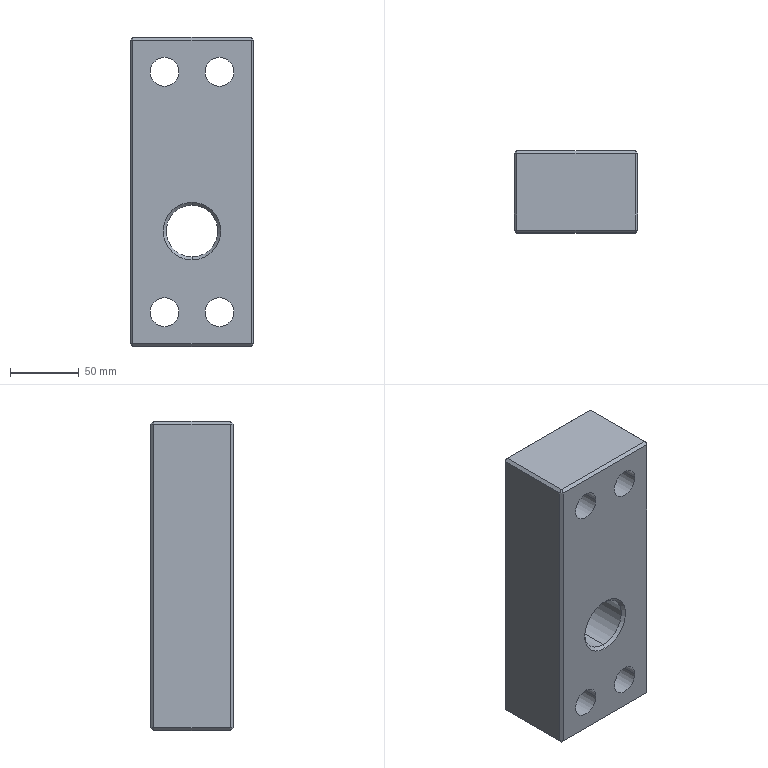Part | Creo | 1 solid | 52 faces | box 90 x 60 x 225 mm | volume 1027341 mm3 | plane 30 | cylinder 18 | cone 4 | commonest cylinder face diameters 21 x8 31 x8 37.616 x2
STEP:
#1=CARTESIAN_POINT('',(43.,400.,103.5));
#2=VERTEX_POINT('',#1);
#3=CARTESIAN_POINT('',(43.,400.,-117.5));
#4=VERTEX_POINT('',#3);
#5=CARTESIAN_POINT('',(43.,400.,103.5));
#6=DIRECTION('',(0.,0.,-1.));
#7=VECTOR('',#6,221.);
#8=LINE('',#5,#7);
#9=EDGE_CURVE('',#2,#4,#8,.T.);
#10=ORIENTED_EDGE('',*,*,#9,.T.);
#11=CARTESIAN_POINT('',(-43.,400.,-117.5));
#12=VERTEX_POINT('',#11);
#13=CARTESIAN_POINT('',(43.,400.,-117.5));
#14=DIRECTION('',(-1.,0.,0.));
#15=VECTOR('',#14,86.);
#16=LINE('',#13,#15);
#17=EDGE_CURVE('',#4,#12,#16,.T.);
#18=ORIENTED_EDGE('',*,*,#17,.T.);
#19=CARTESIAN_POINT('',(-43.,400.,103.5));
#20=VERTEX_POINT('',#19);
#21=CARTESIAN_POINT('',(-43.,400.,-117.5));
#22=DIRECTION('',(0.,0.,1.));
#23=VECTOR('',#22,221.);
#24=LINE('',#21,#23);
#25=EDGE_CURVE('',#12,#20,#24,.T.);
#26=ORIENTED_EDGE('',*,*,#25,.T.);
#27=CARTESIAN_POINT('',(-43.,400.,103.5));
#28=DIRECTION('',(1.,0.,0.));
#29=VECTOR('',#28,86.);
#30=LINE('',#27,#29);
#31=EDGE_CURVE('',#20,#2,#30,.T.);
#32=ORIENTED_EDGE('',*,*,#31,.T.);
#33=EDGE_LOOP('',(#10,#18,#26,#32));
#34=FACE_OUTER_BOUND('',#33,.F.);
#35=CARTESIAN_POINT('',(-30.5,400.,80.5));
#36=VERTEX_POINT('',#35);
#37=CARTESIAN_POINT('',(-9.5,400.,80.5));
#38=VERTEX_POINT('',#37);
#39=CARTESIAN_POINT('',(-20.,400.,80.5));
#40=DIRECTION('',(0.,1.,0.));
#41=DIRECTION('',(-1.,0.,0.));
#42=AXIS2_PLACEMENT_3D('',#39,#40,#41);
#43=CIRCLE('',#42,10.5);
#44=EDGE_CURVE('',#36,#38,#43,.T.);
#45=ORIENTED_EDGE('',*,*,#44,.F.);
#46=CARTESIAN_POINT('',(-20.,400.,80.5));
#47=DIRECTION('',(0.,1.,0.));
#48=DIRECTION('',(1.,0.,0.));
#49=AXIS2_PLACEMENT_3D('',#46,#47,#48);
#50=CIRCLE('',#49,10.5);
#51=EDGE_CURVE('',#38,#36,#50,.T.);
#52=ORIENTED_EDGE('',*,*,#51,.F.);
#53=EDGE_LOOP('',(#45,#52));
#54=FACE_BOUND('',#53,.F.);
#55=CARTESIAN_POINT('',(9.5,400.,-94.5));
#56=VERTEX_POINT('',#55);
#57=CARTESIAN_POINT('',(30.5,400.,-94.5));
#58=VERTEX_POINT('',#57);
#59=CARTESIAN_POINT('',(20.,400.,-94.5));
#60=DIRECTION('',(0.,1.,0.));
#61=DIRECTION('',(-1.,0.,0.));
#62=AXIS2_PLACEMENT_3D('',#59,#60,#61);
#63=CIRCLE('',#62,10.5);
#64=EDGE_CURVE('',#56,#58,#63,.T.);
#65=ORIENTED_EDGE('',*,*,#64,.F.);
#66=CARTESIAN_POINT('',(20.,400.,-94.5));
#67=DIRECTION('',(0.,1.,0.));
#68=DIRECTION('',(1.,0.,0.));
#69=AXIS2_PLACEMENT_3D('',#66,#67,#68);
#70=CIRCLE('',#69,10.5);
#71=EDGE_CURVE('',#58,#56,#70,.T.);
#72=ORIENTED_EDGE('',*,*,#71,.F.);
#73=EDGE_LOOP('',(#65,#72));
#74=FACE_BOUND('',#73,.F.);
#75=CARTESIAN_POINT('',(0.,400.,-56.5));
#76=VERTEX_POINT('',#75);
#77=CARTESIAN_POINT('',(0.,400.,-14.5));
#78=VERTEX_POINT('',#77);
#79=CARTESIAN_POINT('',(0.,400.,-35.5));
#80=DIRECTION('',(0.,1.,0.));
#81=DIRECTION('',(0.,0.,-1.));
#82=AXIS2_PLACEMENT_3D('',#79,#80,#81);
#83=CIRCLE('',#82,21.);
#84=EDGE_CURVE('',#76,#78,#83,.T.);
#85=ORIENTED_EDGE('',*,*,#84,.F.);
#86=CARTESIAN_POINT('',(0.,400.,-35.5));
#87=DIRECTION('',(0.,1.,0.));
#88=DIRECTION('',(0.,0.,1.));
#89=AXIS2_PLACEMENT_3D('',#86,#87,#88);
#90=CIRCLE('',#89,21.);
#91=EDGE_CURVE('',#78,#76,#90,.T.);
#92=ORIENTED_EDGE('',*,*,#91,.F.);
#93=EDGE_LOOP('',(#85,#92));
#94=FACE_BOUND('',#93,.F.);
#95=CARTESIAN_POINT('',(9.5,400.,80.5));
#96=VERTEX_POINT('',#95);
#97=CARTESIAN_POINT('',(30.5,400.,80.5));
#98=VERTEX_POINT('',#97);
#99=CARTESIAN_POINT('',(20.,400.,80.5));
#100=DIRECTION('',(0.,1.,0.));
#101=DIRECTION('',(-1.,0.,0.));
#102=AXIS2_PLACEMENT_3D('',#99,#100,#101);
#103=CIRCLE('',#102,10.5);
#104=EDGE_CURVE('',#96,#98,#103,.T.);
#105=ORIENTED_EDGE('',*,*,#104,.F.);
#106=CARTESIAN_POINT('',(20.,400.,80.5));
#107=DIRECTION('',(0.,1.,0.));
#108=DIRECTION('',(1.,0.,0.));
#109=AXIS2_PLACEMENT_3D('',#106,#107,#108);
#110=CIRCLE('',#109,10.5);
#111=EDGE_CURVE('',#98,#96,#110,.T.);
#112=ORIENTED_EDGE('',*,*,#111,.F.);
#113=EDGE_LOOP('',(#105,#112));
#114=FACE_BOUND('',#113,.F.);
#115=CARTESIAN_POINT('',(-30.5,400.,-94.5));
#116=VERTEX_POINT('',#115);
#117=CARTESIAN_POINT('',(-9.5,400.,-94.5));
#118=VERTEX_POINT('',#117);
#119=CARTESIAN_POINT('',(-20.,400.,-94.5));
#120=DIRECTION('',(0.,1.,0.));
#121=DIRECTION('',(-1.,0.,0.));
#122=AXIS2_PLACEMENT_3D('',#119,#120,#121);
#123=CIRCLE('',#122,10.5);
#124=EDGE_CURVE('',#116,#118,#123,.T.);
#125=ORIENTED_EDGE('',*,*,#124,.F.);
#126=CARTESIAN_POINT('',(-20.,400.,-94.5));
#127=DIRECTION('',(0.,1.,0.));
#128=DIRECTION('',(1.,0.,0.));
#129=AXIS2_PLACEMENT_3D('',#126,#127,#128);
#130=CIRCLE('',#129,10.5);
#131=EDGE_CURVE('',#118,#116,#130,.T.);
#132=ORIENTED_EDGE('',*,*,#131,.F.);
#133=EDGE_LOOP('',(#125,#132));
#134=FACE_BOUND('',#133,.F.);
#135=CARTESIAN_POINT('',(0.,400.,-120.5));
#136=DIRECTION('',(0.,-1.,0.));
#137=DIRECTION('',(0.,0.,-1.));
#138=AXIS2_PLACEMENT_3D('',#135,#136,#137);
#139=PLANE('',#138);
#140=ADVANCED_FACE('',(#34,#54,#74,#94,#114,#134),#139,.T.);
#141=CARTESIAN_POINT('',(30.5,439.,-94.5));
#142=VERTEX_POINT('',#141);
#143=CARTESIAN_POINT('',(9.5,439.,-94.5));
#144=VERTEX_POINT('',#143);
#145=CARTESIAN_POINT('',(20.,439.,-94.5));
#146=DIRECTION('',(0.,-1.,0.));
#147=DIRECTION('',(1.,0.,0.));
#148=AXIS2_PLACEMENT_3D('',#145,#146,#147);
#149=CIRCLE('',#148,10.5);
#150=EDGE_CURVE('',#142,#144,#149,.T.);
#151=ORIENTED_EDGE('',*,*,#150,.T.);
#152=CARTESIAN_POINT('',(9.5,400.,-94.5));
#153=DIRECTION('',(0.,1.,0.));
#154=VECTOR('',#153,39.);
#155=LINE('',#152,#154);
#156=EDGE_CURVE('',#56,#144,#155,.T.);
#157=ORIENTED_EDGE('',*,*,#156,.F.);
#158=ORIENTED_EDGE('',*,*,#64,.T.);
#159=CARTESIAN_POINT('',(30.5,400.,-94.5));
#160=DIRECTION('',(0.,1.,0.));
#161=VECTOR('',#160,39.);
#162=LINE('',#159,#161);
#163=EDGE_CURVE('',#58,#142,#162,.T.);
#164=ORIENTED_EDGE('',*,*,#163,.T.);
#165=EDGE_LOOP('',(#151,#157,#158,#164));
#166=FACE_OUTER_BOUND('',#165,.F.);
#167=CARTESIAN_POINT('',(20.,400.,-94.5));
#168=DIRECTION('',(0.,1.,0.));
#169=DIRECTION('',(-1.,0.,0.));
#170=AXIS2_PLACEMENT_3D('',#167,#168,#169);
#171=CYLINDRICAL_SURFACE('',#170,10.5);
#172=ADVANCED_FACE('',(#166),#171,.F.);
#173=CARTESIAN_POINT('',(4.5,439.,-94.5));
#174=VERTEX_POINT('',#173);
#175=CARTESIAN_POINT('',(35.5,439.,-94.5));
#176=VERTEX_POINT('',#175);
#177=CARTESIAN_POINT('',(20.,439.,-94.5));
#178=DIRECTION('',(0.,1.,0.));
#179=DIRECTION('',(-1.,0.,0.));
#180=AXIS2_PLACEMENT_3D('',#177,#178,#179);
#181=CIRCLE('',#180,15.5);
#182=EDGE_CURVE('',#174,#176,#181,.T.);
#183=ORIENTED_EDGE('',*,*,#182,.F.);
#184=CARTESIAN_POINT('',(20.,439.,-94.5));
#185=DIRECTION('',(0.,1.,0.));
#186=DIRECTION('',(1.,0.,0.));
#187=AXIS2_PLACEMENT_3D('',#184,#185,#186);
#188=CIRCLE('',#187,15.5);
#189=EDGE_CURVE('',#176,#174,#188,.T.);
#190=ORIENTED_EDGE('',*,*,#189,.F.);
#191=EDGE_LOOP('',(#183,#190));
#192=FACE_OUTER_BOUND('',#191,.F.);
#193=CARTESIAN_POINT('',(20.,439.,-94.5));
#194=DIRECTION('',(0.,-1.,0.));
#195=DIRECTION('',(-1.,0.,0.));
#196=AXIS2_PLACEMENT_3D('',#193,#194,#195);
#197=CIRCLE('',#196,10.5);
#198=EDGE_CURVE('',#144,#142,#197,.T.);
#199=ORIENTED_EDGE('',*,*,#198,.F.);
#200=ORIENTED_EDGE('',*,*,#150,.F.);
#201=EDGE_LOOP('',(#199,#200));
#202=FACE_BOUND('',#201,.F.);
#203=CARTESIAN_POINT('',(20.,439.,-94.5));
#204=DIRECTION('',(0.,-1.,0.));
#205=DIRECTION('',(1.,0.,0.));
#206=AXIS2_PLACEMENT_3D('',#203,#204,#205);
#207=PLANE('',#206);
#208=ADVANCED_FACE('',(#192,#202),#207,.F.);
#209=ORIENTED_EDGE('',*,*,#198,.T.);
#210=ORIENTED_EDGE('',*,*,#163,.F.);
#211=ORIENTED_EDGE('',*,*,#71,.T.);
#212=ORIENTED_EDGE('',*,*,#156,.T.);
#213=EDGE_LOOP('',(#209,#210,#211,#212));
#214=FACE_OUTER_BOUND('',#213,.F.);
#215=CARTESIAN_POINT('',(20.,400.,-94.5));
#216=DIRECTION('',(0.,1.,0.));
#217=DIRECTION('',(-1.,0.,0.));
#218=AXIS2_PLACEMENT_3D('',#215,#216,#217);
#219=CYLINDRICAL_SURFACE('',#218,10.5);
#220=ADVANCED_FACE('',(#214),#219,.F.);
#221=CARTESIAN_POINT('',(35.5,460.,-94.5));
#222=VERTEX_POINT('',#221);
#223=CARTESIAN_POINT('',(4.5,460.,-94.5));
#224=VERTEX_POINT('',#223);
#225=CARTESIAN_POINT('',(20.,460.,-94.5));
#226=DIRECTION('',(0.,-1.,0.));
#227=DIRECTION('',(1.,0.,0.));
#228=AXIS2_PLACEMENT_3D('',#225,#226,#227);
#229=CIRCLE('',#228,15.5);
#230=EDGE_CURVE('',#222,#224,#229,.T.);
#231=ORIENTED_EDGE('',*,*,#230,.T.);
#232=CARTESIAN_POINT('',(4.5,439.,-94.5));
#233=DIRECTION('',(0.,1.,0.));
#234=VECTOR('',#233,21.);
#235=LINE('',#232,#234);
#236=EDGE_CURVE('',#174,#224,#235,.T.);
#237=ORIENTED_EDGE('',*,*,#236,.F.);
#238=ORIENTED_EDGE('',*,*,#182,.T.);
#239=CARTESIAN_POINT('',(35.5,439.,-94.5));
#240=DIRECTION('',(0.,1.,0.));
#241=VECTOR('',#240,21.);
#242=LINE('',#239,#241);
#243=EDGE_CURVE('',#176,#222,#242,.T.);
#244=ORIENTED_EDGE('',*,*,#243,.T.);
#245=EDGE_LOOP('',(#231,#237,#238,#244));
#246=FACE_OUTER_BOUND('',#245,.F.);
#247=CARTESIAN_POINT('',(20.,439.,-94.5));
#248=DIRECTION('',(0.,1.,0.));
#249=DIRECTION('',(-1.,0.,0.));
#250=AXIS2_PLACEMENT_3D('',#247,#248,#249);
#251=CYLINDRICAL_SURFACE('',#250,15.5);
#252=ADVANCED_FACE('',(#246),#251,.F.);
#253=CARTESIAN_POINT('',(43.,460.,-117.5));
#254=VERTEX_POINT('',#253);
#255=CARTESIAN_POINT('',(43.,460.,103.5));
#256=VERTEX_POINT('',#255);
#257=CARTESIAN_POINT('',(43.,460.,-117.5));
#258=DIRECTION('',(0.,0.,1.));
#259=VECTOR('',#258,221.);
#260=LINE('',#257,#259);
#261=EDGE_CURVE('',#254,#256,#260,.T.);
#262=ORIENTED_EDGE('',*,*,#261,.T.);
#263=CARTESIAN_POINT('',(-43.,460.,103.5));
#264=VERTEX_POINT('',#263);
#265=CARTESIAN_POINT('',(43.,460.,103.5));
#266=DIRECTION('',(-1.,0.,0.));
#267=VECTOR('',#266,86.);
#268=LINE('',#265,#267);
#269=EDGE_CURVE('',#256,#264,#268,.T.);
#270=ORIENTED_EDGE('',*,*,#269,.T.);
#271=CARTESIAN_POINT('',(-43.,460.,-117.5));
#272=VERTEX_POINT('',#271);
#273=CARTESIAN_POINT('',(-43.,460.,103.5));
#274=DIRECTION('',(0.,0.,-1.));
#275=VECTOR('',#274,221.);
#276=LINE('',#273,#275);
#277=EDGE_CURVE('',#264,#272,#276,.T.);
#278=ORIENTED_EDGE('',*,*,#277,.T.);
#279=CARTESIAN_POINT('',(-43.,460.,-117.5));
#280=DIRECTION('',(1.,0.,0.));
#281=VECTOR('',#280,86.);
#282=LINE('',#279,#281);
#283=EDGE_CURVE('',#272,#254,#282,.T.);
#284=ORIENTED_EDGE('',*,*,#283,.T.);
#285=EDGE_LOOP('',(#262,#270,#278,#284));
#286=FACE_OUTER_BOUND('',#285,.F.);
#287=CARTESIAN_POINT('',(20.,460.,-94.5));
#288=DIRECTION('',(0.,-1.,0.));
#289=DIRECTION('',(-1.,0.,0.));
#290=AXIS2_PLACEMENT_3D('',#287,#288,#289);
#291=CIRCLE('',#290,15.5);
#292=EDGE_CURVE('',#224,#222,#291,.T.);
#293=ORIENTED_EDGE('',*,*,#292,.F.);
#294=ORIENTED_EDGE('',*,*,#230,.F.);
#295=EDGE_LOOP('',(#293,#294));
#296=FACE_BOUND('',#295,.F.);
#297=CARTESIAN_POINT('',(4.5,460.,80.5));
#298=VERTEX_POINT('',#297);
#299=CARTESIAN_POINT('',(35.5,460.,80.5));
#300=VERTEX_POINT('',#299);
#301=CARTESIAN_POINT('',(20.,460.,80.5));
#302=DIRECTION('',(0.,-1.,0.));
#303=DIRECTION('',(-1.,0.,0.));
#304=AXIS2_PLACEMENT_3D('',#301,#302,#303);
#305=CIRCLE('',#304,15.5);
#306=EDGE_CURVE('',#298,#300,#305,.T.);
#307=ORIENTED_EDGE('',*,*,#306,.F.);
#308=CARTESIAN_POINT('',(20.,460.,80.5));
#309=DIRECTION('',(0.,-1.,0.));
#310=DIRECTION('',(1.,0.,0.));
#311=AXIS2_PLACEMENT_3D('',#308,#309,#310);
#312=CIRCLE('',#311,15.5);
#313=EDGE_CURVE('',#300,#298,#312,.T.);
#314=ORIENTED_EDGE('',*,*,#313,.F.);
#315=EDGE_LOOP('',(#307,#314));
#316=FACE_BOUND('',#315,.F.);
#317=CARTESIAN_POINT('',(-35.5,460.,80.5));
#318=VERTEX_POINT('',#317);
#319=CARTESIAN_POINT('',(-4.5,460.,80.5));
#320=VERTEX_POINT('',#319);
#321=CARTESIAN_POINT('',(-20.,460.,80.5));
#322=DIRECTION('',(0.,-1.,0.));
#323=DIRECTION('',(-1.,0.,0.));
#324=AXIS2_PLACEMENT_3D('',#321,#322,#323);
#325=CIRCLE('',#324,15.5);
#326=EDGE_CURVE('',#318,#320,#325,.T.);
#327=ORIENTED_EDGE('',*,*,#326,.F.);
#328=CARTESIAN_POINT('',(-20.,460.,80.5));
#329=DIRECTION('',(0.,-1.,0.));
#330=DIRECTION('',(1.,0.,0.));
#331=AXIS2_PLACEMENT_3D('',#328,#329,#330);
#332=CIRCLE('',#331,15.5);
#333=EDGE_CURVE('',#320,#318,#332,.T.);
#334=ORIENTED_EDGE('',*,*,#333,.F.);
#335=EDGE_LOOP('',(#327,#334));
#336=FACE_BOUND('',#335,.F.);
#337=CARTESIAN_POINT('',(-35.5,460.,-94.5));
#338=VERTEX_POINT('',#337);
#339=CARTESIAN_POINT('',(-4.5,460.,-94.5));
#340=VERTEX_POINT('',#339);
#341=CARTESIAN_POINT('',(-20.,460.,-94.5));
#342=DIRECTION('',(0.,-1.,0.));
#343=DIRECTION('',(-1.,0.,0.));
#344=AXIS2_PLACEMENT_3D('',#341,#342,#343);
#345=CIRCLE('',#344,15.5);
#346=EDGE_CURVE('',#338,#340,#345,.T.);
#347=ORIENTED_EDGE('',*,*,#346,.F.);
#348=CARTESIAN_POINT('',(-20.,460.,-94.5));
#349=DIRECTION('',(0.,-1.,0.));
#350=DIRECTION('',(1.,0.,0.));
#351=AXIS2_PLACEMENT_3D('',#348,#349,#350);
#352=CIRCLE('',#351,15.5);
#353=EDGE_CURVE('',#340,#338,#352,.T.);
#354=ORIENTED_EDGE('',*,*,#353,.F.);
#355=EDGE_LOOP('',(#347,#354));
#356=FACE_BOUND('',#355,.F.);
#357=CARTESIAN_POINT('',(0.,460.,-14.5));
#358=VERTEX_POINT('',#357);
#359=CARTESIAN_POINT('',(0.,460.,-56.5));
#360=VERTEX_POINT('',#359);
#361=CARTESIAN_POINT('',(0.,460.,-35.5));
#362=DIRECTION('',(0.,-1.,0.));
#363=DIRECTION('',(0.,0.,1.));
#364=AXIS2_PLACEMENT_3D('',#361,#362,#363);
#365=CIRCLE('',#364,21.);
#366=EDGE_CURVE('',#358,#360,#365,.T.);
#367=ORIENTED_EDGE('',*,*,#366,.F.);
#368=CARTESIAN_POINT('',(0.,460.,-35.5));
#369=DIRECTION('',(0.,-1.,0.));
#370=DIRECTION('',(0.,0.,-1.));
#371=AXIS2_PLACEMENT_3D('',#368,#369,#370);
#372=CIRCLE('',#371,21.);
#373=EDGE_CURVE('',#360,#358,#372,.T.);
#374=ORIENTED_EDGE('',*,*,#373,.F.);
#375=EDGE_LOOP('',(#367,#374));
#376=FACE_BOUND('',#375,.F.);
#377=CARTESIAN_POINT('',(0.,460.,-120.5));
#378=DIRECTION('',(0.,1.,0.));
#379=DIRECTION('',(0.,0.,1.));
#380=AXIS2_PLACEMENT_3D('',#377,#378,#379);
#381=PLANE('',#380);
#382=ADVANCED_FACE('',(#286,#296,#316,#336,#356,#376),#381,.T.);
#383=ORIENTED_EDGE('',*,*,#346,.T.);
#384=CARTESIAN_POINT('',(-4.5,439.,-94.5));
#385=VERTEX_POINT('',#384);
#386=CARTESIAN_POINT('',(-4.5,439.,-94.5));
#387=DIRECTION('',(0.,1.,0.));
#388=VECTOR('',#387,21.);
#389=LINE('',#386,#388);
#390=EDGE_CURVE('',#385,#340,#389,.T.);
#391=ORIENTED_EDGE('',*,*,#390,.F.);
#392=CARTESIAN_POINT('',(-35.5,439.,-94.5));
#393=VERTEX_POINT('',#392);
#394=CARTESIAN_POINT('',(-20.,439.,-94.5));
#395=DIRECTION('',(0.,1.,0.));
#396=DIRECTION('',(1.,0.,0.));
#397=AXIS2_PLACEMENT_3D('',#394,#395,#396);
#398=CIRCLE('',#397,15.5);
#399=EDGE_CURVE('',#385,#393,#398,.T.);
#400=ORIENTED_EDGE('',*,*,#399,.T.);
#401=CARTESIAN_POINT('',(-35.5,439.,-94.5));
#402=DIRECTION('',(0.,1.,0.));
#403=VECTOR('',#402,21.);
#404=LINE('',#401,#403);
#405=EDGE_CURVE('',#393,#338,#404,.T.);
#406=ORIENTED_EDGE('',*,*,#405,.T.);
#407=EDGE_LOOP('',(#383,#391,#400,#406));
#408=FACE_OUTER_BOUND('',#407,.F.);
#409=CARTESIAN_POINT('',(-20.,439.,-94.5));
#410=DIRECTION('',(0.,1.,0.));
#411=DIRECTION('',(-1.,0.,0.));
#412=AXIS2_PLACEMENT_3D('',#409,#410,#411);
#413=CYLINDRICAL_SURFACE('',#412,15.5);
#414=ADVANCED_FACE('',(#408),#413,.F.);
#415=ORIENTED_EDGE('',*,*,#353,.T.);
#416=ORIENTED_EDGE('',*,*,#405,.F.);
#417=CARTESIAN_POINT('',(-20.,439.,-94.5));
#418=DIRECTION('',(0.,1.,0.));
#419=DIRECTION('',(-1.,0.,0.));
#420=AXIS2_PLACEMENT_3D('',#417,#418,#419);
#421=CIRCLE('',#420,15.5);
#422=EDGE_CURVE('',#393,#385,#421,.T.);
#423=ORIENTED_EDGE('',*,*,#422,.T.);
#424=ORIENTED_EDGE('',*,*,#390,.T.);
#425=EDGE_LOOP('',(#415,#416,#423,#424));
#426=FACE_OUTER_BOUND('',#425,.F.);
#427=CARTESIAN_POINT('',(-20.,439.,-94.5));
#428=DIRECTION('',(0.,1.,0.));
#429=DIRECTION('',(-1.,0.,0.));
#430=AXIS2_PLACEMENT_3D('',#427,#428,#429);
#431=CYLINDRICAL_SURFACE('',#430,15.5);
#432=ADVANCED_FACE('',(#426),#431,.F.);
#433=ORIENTED_EDGE('',*,*,#422,.F.);
#434=ORIENTED_EDGE('',*,*,#399,.F.);
#435=EDGE_LOOP('',(#433,#434));
#436=FACE_OUTER_BOUND('',#435,.F.);
#437=CARTESIAN_POINT('',(-30.5,439.,-94.5));
#438=VERTEX_POINT('',#437);
#439=CARTESIAN_POINT('',(-9.5,439.,-94.5));
#440=VERTEX_POINT('',#439);
#441=CARTESIAN_POINT('',(-20.,439.,-94.5));
#442=DIRECTION('',(0.,-1.,0.));
#443=DIRECTION('',(-1.,0.,0.));
#444=AXIS2_PLACEMENT_3D('',#441,#442,#443);
#445=CIRCLE('',#444,10.5);
#446=EDGE_CURVE('',#438,#440,#445,.T.);
#447=ORIENTED_EDGE('',*,*,#446,.F.);
#448=CARTESIAN_POINT('',(-20.,439.,-94.5));
#449=DIRECTION('',(0.,-1.,0.));
#450=DIRECTION('',(1.,0.,0.));
#451=AXIS2_PLACEMENT_3D('',#448,#449,#450);
#452=CIRCLE('',#451,10.5);
#453=EDGE_CURVE('',#440,#438,#452,.T.);
#454=ORIENTED_EDGE('',*,*,#453,.F.);
#455=EDGE_LOOP('',(#447,#454));
#456=FACE_BOUND('',#455,.F.);
#457=CARTESIAN_POINT('',(-20.,439.,-94.5));
#458=DIRECTION('',(0.,-1.,0.));
#459=DIRECTION('',(1.,0.,0.));
#460=AXIS2_PLACEMENT_3D('',#457,#458,#459);
#461=PLANE('',#460);
#462=ADVANCED_FACE('',(#436,#456),#461,.F.);
#463=ORIENTED_EDGE('',*,*,#446,.T.);
#464=CARTESIAN_POINT('',(-9.5,400.,-94.5));
#465=DIRECTION('',(0.,1.,0.));
#466=VECTOR('',#465,39.);
#467=LINE('',#464,#466);
#468=EDGE_CURVE('',#118,#440,#467,.T.);
#469=ORIENTED_EDGE('',*,*,#468,.F.);
#470=ORIENTED_EDGE('',*,*,#131,.T.);
#471=CARTESIAN_POINT('',(-30.5,400.,-94.5));
#472=DIRECTION('',(0.,1.,0.));
#473=VECTOR('',#472,39.);
#474=LINE('',#471,#473);
#475=EDGE_CURVE('',#116,#438,#474,.T.);
#476=ORIENTED_EDGE('',*,*,#475,.T.);
#477=EDGE_LOOP('',(#463,#469,#470,#476));
#478=FACE_OUTER_BOUND('',#477,.F.);
#479=CARTESIAN_POINT('',(-20.,400.,-94.5));
#480=DIRECTION('',(0.,1.,0.));
#481=DIRECTION('',(-1.,0.,0.));
#482=AXIS2_PLACEMENT_3D('',#479,#480,#481);
#483=CYLINDRICAL_SURFACE('',#482,10.5);
#484=ADVANCED_FACE('',(#478),#483,.F.);
#485=ORIENTED_EDGE('',*,*,#453,.T.);
#486=ORIENTED_EDGE('',*,*,#475,.F.);
#487=ORIENTED_EDGE('',*,*,#124,.T.);
#488=ORIENTED_EDGE('',*,*,#468,.T.);
#489=EDGE_LOOP('',(#485,#486,#487,#488));
#490=FACE_OUTER_BOUND('',#489,.F.);
#491=CARTESIAN_POINT('',(-20.,400.,-94.5));
#492=DIRECTION('',(0.,1.,0.));
#493=DIRECTION('',(-1.,0.,0.));
#494=AXIS2_PLACEMENT_3D('',#491,#492,#493);
#495=CYLINDRICAL_SURFACE('',#494,10.5);
#496=ADVANCED_FACE('',(#490),#495,.F.);
#497=ORIENTED_EDGE('',*,*,#292,.T.);
#498=ORIENTED_EDGE('',*,*,#243,.F.);
#499=ORIENTED_EDGE('',*,*,#189,.T.);
#500=ORIENTED_EDGE('',*,*,#236,.T.);
#501=EDGE_LOOP('',(#497,#498,#499,#500));
#502=FACE_OUTER_BOUND('',#501,.F.);
#503=CARTESIAN_POINT('',(20.,439.,-94.5));
#504=DIRECTION('',(0.,1.,0.));
#505=DIRECTION('',(-1.,0.,0.));
#506=AXIS2_PLACEMENT_3D('',#503,#504,#505);
#507=CYLINDRICAL_SURFACE('',#506,15.5);
#508=ADVANCED_FACE('',(#502),#507,.F.);
#509=ORIENTED_EDGE('',*,*,#306,.T.);
#510=CARTESIAN_POINT('',(35.5,439.,80.5));
#511=VERTEX_POINT('',#510);
#512=CARTESIAN_POINT('',(35.5,439.,80.5));
#513=DIRECTION('',(0.,1.,0.));
#514=VECTOR('',#513,21.);
#515=LINE('',#512,#514);
#516=EDGE_CURVE('',#511,#300,#515,.T.);
#517=ORIENTED_EDGE('',*,*,#516,.F.);
#518=CARTESIAN_POINT('',(4.5,439.,80.5));
#519=VERTEX_POINT('',#518);
#520=CARTESIAN_POINT('',(20.,439.,80.5));
#521=DIRECTION('',(0.,1.,0.));
#522=DIRECTION('',(1.,0.,0.));
#523=AXIS2_PLACEMENT_3D('',#520,#521,#522);
#524=CIRCLE('',#523,15.5);
#525=EDGE_CURVE('',#511,#519,#524,.T.);
#526=ORIENTED_EDGE('',*,*,#525,.T.);
#527=CARTESIAN_POINT('',(4.5,439.,80.5));
#528=DIRECTION('',(0.,1.,0.));
#529=VECTOR('',#528,21.);
#530=LINE('',#527,#529);
#531=EDGE_CURVE('',#519,#298,#530,.T.);
#532=ORIENTED_EDGE('',*,*,#531,.T.);
#533=EDGE_LOOP('',(#509,#517,#526,#532));
#534=FACE_OUTER_BOUND('',#533,.F.);
#535=CARTESIAN_POINT('',(20.,439.,80.5));
#536=DIRECTION('',(0.,1.,0.));
#537=DIRECTION('',(-1.,0.,0.));
#538=AXIS2_PLACEMENT_3D('',#535,#536,#537);
#539=CYLINDRICAL_SURFACE('',#538,15.5);
#540=ADVANCED_FACE('',(#534),#539,.F.);
#541=ORIENTED_EDGE('',*,*,#313,.T.);
#542=ORIENTED_EDGE('',*,*,#531,.F.);
#543=CARTESIAN_POINT('',(20.,439.,80.5));
#544=DIRECTION('',(0.,1.,0.));
#545=DIRECTION('',(-1.,0.,0.));
#546=AXIS2_PLACEMENT_3D('',#543,#544,#545);
#547=CIRCLE('',#546,15.5);
#548=EDGE_CURVE('',#519,#511,#547,.T.);
#549=ORIENTED_EDGE('',*,*,#548,.T.);
#550=ORIENTED_EDGE('',*,*,#516,.T.);
#551=EDGE_LOOP('',(#541,#542,#549,#550));
#552=FACE_OUTER_BOUND('',#551,.F.);
#553=CARTESIAN_POINT('',(20.,439.,80.5));
#554=DIRECTION('',(0.,1.,0.));
#555=DIRECTION('',(-1.,0.,0.));
#556=AXIS2_PLACEMENT_3D('',#553,#554,#555);
#557=CYLINDRICAL_SURFACE('',#556,15.5);
#558=ADVANCED_FACE('',(#552),#557,.F.);
#559=ORIENTED_EDGE('',*,*,#548,.F.);
#560=ORIENTED_EDGE('',*,*,#525,.F.);
#561=EDGE_LOOP('',(#559,#560));
#562=FACE_OUTER_BOUND('',#561,.F.);
#563=CARTESIAN_POINT('',(9.5,439.,80.5));
#564=VERTEX_POINT('',#563);
#565=CARTESIAN_POINT('',(30.5,439.,80.5));
#566=VERTEX_POINT('',#565);
#567=CARTESIAN_POINT('',(20.,439.,80.5));
#568=DIRECTION('',(0.,-1.,0.));
#569=DIRECTION('',(-1.,0.,0.));
#570=AXIS2_PLACEMENT_3D('',#567,#568,#569);
#571=CIRCLE('',#570,10.5);
#572=EDGE_CURVE('',#564,#566,#571,.T.);
#573=ORIENTED_EDGE('',*,*,#572,.F.);
#574=CARTESIAN_POINT('',(20.,439.,80.5));
#575=DIRECTION('',(0.,-1.,0.));
#576=DIRECTION('',(1.,0.,0.));
#577=AXIS2_PLACEMENT_3D('',#574,#575,#576);
#578=CIRCLE('',#577,10.5);
#579=EDGE_CURVE('',#566,#564,#578,.T.);
#580=ORIENTED_EDGE('',*,*,#579,.F.);
#581=EDGE_LOOP('',(#573,#580));
#582=FACE_BOUND('',#581,.F.);
#583=CARTESIAN_POINT('',(20.,439.,80.5));
#584=DIRECTION('',(0.,-1.,0.));
#585=DIRECTION('',(1.,0.,0.));
#586=AXIS2_PLACEMENT_3D('',#583,#584,#585);
#587=PLANE('',#586);
#588=ADVANCED_FACE('',(#562,#582),#587,.F.);
#589=ORIENTED_EDGE('',*,*,#572,.T.);
#590=CARTESIAN_POINT('',(30.5,400.,80.5));
#591=DIRECTION('',(0.,1.,0.));
#592=VECTOR('',#591,39.);
#593=LINE('',#590,#592);
#594=EDGE_CURVE('',#98,#566,#593,.T.);
#595=ORIENTED_EDGE('',*,*,#594,.F.);
#596=ORIENTED_EDGE('',*,*,#111,.T.);
#597=CARTESIAN_POINT('',(9.5,400.,80.5));
#598=DIRECTION('',(0.,1.,0.));
#599=VECTOR('',#598,39.);
#600=LINE('',#597,#599);
#601=EDGE_CURVE('',#96,#564,#600,.T.);
#602=ORIENTED_EDGE('',*,*,#601,.T.);
#603=EDGE_LOOP('',(#589,#595,#596,#602));
#604=FACE_OUTER_BOUND('',#603,.F.);
#605=CARTESIAN_POINT('',(20.,400.,80.5));
#606=DIRECTION('',(0.,1.,0.));
#607=DIRECTION('',(-1.,0.,0.));
#608=AXIS2_PLACEMENT_3D('',#605,#606,#607);
#609=CYLINDRICAL_SURFACE('',#608,10.5);
#610=ADVANCED_FACE('',(#604),#609,.F.);
#611=ORIENTED_EDGE('',*,*,#579,.T.);
#612=ORIENTED_EDGE('',*,*,#601,.F.);
#613=ORIENTED_EDGE('',*,*,#104,.T.);
#614=ORIENTED_EDGE('',*,*,#594,.T.);
#615=EDGE_LOOP('',(#611,#612,#613,#614));
#616=FACE_OUTER_BOUND('',#615,.F.);
#617=CARTESIAN_POINT('',(20.,400.,80.5));
#618=DIRECTION('',(0.,1.,0.));
#619=DIRECTION('',(-1.,0.,0.));
#620=AXIS2_PLACEMENT_3D('',#617,#618,#619);
#621=CYLINDRICAL_SURFACE('',#620,10.5);
#622=ADVANCED_FACE('',(#616),#621,.F.);
#623=ORIENTED_EDGE('',*,*,#326,.T.);
#624=CARTESIAN_POINT('',(-4.5,439.,80.5));
#625=VERTEX_POINT('',#624);
#626=CARTESIAN_POINT('',(-4.5,439.,80.5));
#627=DIRECTION('',(0.,1.,0.));
#628=VECTOR('',#627,21.);
#629=LINE('',#626,#628);
#630=EDGE_CURVE('',#625,#320,#629,.T.);
#631=ORIENTED_EDGE('',*,*,#630,.F.);
#632=CARTESIAN_POINT('',(-35.5,439.,80.5));
#633=VERTEX_POINT('',#632);
#634=CARTESIAN_POINT('',(-20.,439.,80.5));
#635=DIRECTION('',(0.,1.,0.));
#636=DIRECTION('',(1.,0.,0.));
#637=AXIS2_PLACEMENT_3D('',#634,#635,#636);
#638=CIRCLE('',#637,15.5);
#639=EDGE_CURVE('',#625,#633,#638,.T.);
#640=ORIENTED_EDGE('',*,*,#639,.T.);
#641=CARTESIAN_POINT('',(-35.5,439.,80.5));
#642=DIRECTION('',(0.,1.,0.));
#643=VECTOR('',#642,21.);
#644=LINE('',#641,#643);
#645=EDGE_CURVE('',#633,#318,#644,.T.);
#646=ORIENTED_EDGE('',*,*,#645,.T.);
#647=EDGE_LOOP('',(#623,#631,#640,#646));
#648=FACE_OUTER_BOUND('',#647,.F.);
#649=CARTESIAN_POINT('',(-20.,439.,80.5));
#650=DIRECTION('',(0.,1.,0.));
#651=DIRECTION('',(-1.,0.,0.));
#652=AXIS2_PLACEMENT_3D('',#649,#650,#651);
#653=CYLINDRICAL_SURFACE('',#652,15.5);
#654=ADVANCED_FACE('',(#648),#653,.F.);
#655=ORIENTED_EDGE('',*,*,#333,.T.);
#656=ORIENTED_EDGE('',*,*,#645,.F.);
#657=CARTESIAN_POINT('',(-20.,439.,80.5));
#658=DIRECTION('',(0.,1.,0.));
#659=DIRECTION('',(-1.,0.,0.));
#660=AXIS2_PLACEMENT_3D('',#657,#658,#659);
#661=CIRCLE('',#660,15.5);
#662=EDGE_CURVE('',#633,#625,#661,.T.);
#663=ORIENTED_EDGE('',*,*,#662,.T.);
#664=ORIENTED_EDGE('',*,*,#630,.T.);
#665=EDGE_LOOP('',(#655,#656,#663,#664));
#666=FACE_OUTER_BOUND('',#665,.F.);
#667=CARTESIAN_POINT('',(-20.,439.,80.5));
#668=DIRECTION('',(0.,1.,0.));
#669=DIRECTION('',(-1.,0.,0.));
#670=AXIS2_PLACEMENT_3D('',#667,#668,#669);
#671=CYLINDRICAL_SURFACE('',#670,15.5);
#672=ADVANCED_FACE('',(#666),#671,.F.);
#673=ORIENTED_EDGE('',*,*,#662,.F.);
#674=ORIENTED_EDGE('',*,*,#639,.F.);
#675=EDGE_LOOP('',(#673,#674));
#676=FACE_OUTER_BOUND('',#675,.F.);
#677=CARTESIAN_POINT('',(-30.5,439.,80.5));
#678=VERTEX_POINT('',#677);
#679=CARTESIAN_POINT('',(-9.5,439.,80.5));
#680=VERTEX_POINT('',#679);
#681=CARTESIAN_POINT('',(-20.,439.,80.5));
#682=DIRECTION('',(0.,-1.,0.));
#683=DIRECTION('',(-1.,0.,0.));
#684=AXIS2_PLACEMENT_3D('',#681,#682,#683);
#685=CIRCLE('',#684,10.5);
#686=EDGE_CURVE('',#678,#680,#685,.T.);
#687=ORIENTED_EDGE('',*,*,#686,.F.);
#688=CARTESIAN_POINT('',(-20.,439.,80.5));
#689=DIRECTION('',(0.,-1.,0.));
#690=DIRECTION('',(1.,0.,0.));
#691=AXIS2_PLACEMENT_3D('',#688,#689,#690);
#692=CIRCLE('',#691,10.5);
#693=EDGE_CURVE('',#680,#678,#692,.T.);
#694=ORIENTED_EDGE('',*,*,#693,.F.);
#695=EDGE_LOOP('',(#687,#694));
#696=FACE_BOUND('',#695,.F.);
#697=CARTESIAN_POINT('',(-20.,439.,80.5));
#698=DIRECTION('',(0.,-1.,0.));
#699=DIRECTION('',(1.,0.,0.));
#700=AXIS2_PLACEMENT_3D('',#697,#698,#699);
#701=PLANE('',#700);
#702=ADVANCED_FACE('',(#676,#696),#701,.F.);
#703=ORIENTED_EDGE('',*,*,#686,.T.);
#704=CARTESIAN_POINT('',(-9.5,400.,80.5));
#705=DIRECTION('',(0.,1.,0.));
#706=VECTOR('',#705,39.);
#707=LINE('',#704,#706);
#708=EDGE_CURVE('',#38,#680,#707,.T.);
#709=ORIENTED_EDGE('',*,*,#708,.F.);
#710=ORIENTED_EDGE('',*,*,#51,.T.);
#711=CARTESIAN_POINT('',(-30.5,400.,80.5));
#712=DIRECTION('',(0.,1.,0.));
#713=VECTOR('',#712,39.);
#714=LINE('',#711,#713);
#715=EDGE_CURVE('',#36,#678,#714,.T.);
#716=ORIENTED_EDGE('',*,*,#715,.T.);
#717=EDGE_LOOP('',(#703,#709,#710,#716));
#718=FACE_OUTER_BOUND('',#717,.F.);
#719=CARTESIAN_POINT('',(-20.,400.,80.5));
#720=DIRECTION('',(0.,1.,0.));
#721=DIRECTION('',(-1.,0.,0.));
#722=AXIS2_PLACEMENT_3D('',#719,#720,#721);
#723=CYLINDRICAL_SURFACE('',#722,10.5);
#724=ADVANCED_FACE('',(#718),#723,.F.);
#725=ORIENTED_EDGE('',*,*,#693,.T.);
#726=ORIENTED_EDGE('',*,*,#715,.F.);
#727=ORIENTED_EDGE('',*,*,#44,.T.);
#728=ORIENTED_EDGE('',*,*,#708,.T.);
#729=EDGE_LOOP('',(#725,#726,#727,#728));
#730=FACE_OUTER_BOUND('',#729,.F.);
#731=CARTESIAN_POINT('',(-20.,400.,80.5));
#732=DIRECTION('',(0.,1.,0.));
#733=DIRECTION('',(-1.,0.,0.));
#734=AXIS2_PLACEMENT_3D('',#731,#732,#733);
#735=CYLINDRICAL_SURFACE('',#734,10.5);
#736=ADVANCED_FACE('',(#730),#735,.F.);
#737=CARTESIAN_POINT('',(45.,458.,-117.5));
#738=VERTEX_POINT('',#737);
#739=CARTESIAN_POINT('',(43.,460.,-117.5));
#740=DIRECTION('',(0.7071,-0.7071,0.));
#741=VECTOR('',#740,2.828);
#742=LINE('',#739,#741);
#743=EDGE_CURVE('',#254,#738,#742,.T.);
#744=ORIENTED_EDGE('',*,*,#743,.T.);
#745=CARTESIAN_POINT('',(45.,458.,103.5));
#746=VERTEX_POINT('',#745);
#747=CARTESIAN_POINT('',(45.,458.,103.5));
#748=DIRECTION('',(0.,0.,-1.));
#749=VECTOR('',#748,221.);
#750=LINE('',#747,#749);
#751=EDGE_CURVE('',#746,#738,#750,.T.);
#752=ORIENTED_EDGE('',*,*,#751,.F.);
#753=CARTESIAN_POINT('',(45.,458.,103.5));
#754=DIRECTION('',(-0.7071,0.7071,0.));
#755=VECTOR('',#754,2.828);
#756=LINE('',#753,#755);
#757=EDGE_CURVE('',#746,#256,#756,.T.);
#758=ORIENTED_EDGE('',*,*,#757,.T.);
#759=ORIENTED_EDGE('',*,*,#261,.F.);
#760=EDGE_LOOP('',(#744,#752,#758,#759));
#761=FACE_OUTER_BOUND('',#760,.F.);
#762=CARTESIAN_POINT('',(43.,460.,-120.5));
#763=DIRECTION('',(-0.7071,-0.7071,0.));
#764=DIRECTION('',(0.7071,-0.7071,0.));
#765=AXIS2_PLACEMENT_3D('',#762,#763,#764);
#766=PLANE('',#765);
#767=ADVANCED_FACE('',(#761),#766,.F.);
#768=CARTESIAN_POINT('',(43.,458.,-119.5));
#769=VERTEX_POINT('',#768);
#770=CARTESIAN_POINT('',(45.,458.,-117.5));
#771=DIRECTION('',(-0.7071,0.,-0.7071));
#772=VECTOR('',#771,2.828);
#773=LINE('',#770,#772);
#774=EDGE_CURVE('',#738,#769,#773,.T.);
#775=ORIENTED_EDGE('',*,*,#774,.F.);
#776=ORIENTED_EDGE('',*,*,#743,.F.);
#777=CARTESIAN_POINT('',(43.,458.,-119.5));
#778=DIRECTION('',(0.,0.7071,0.7071));
#779=VECTOR('',#778,2.828);
#780=LINE('',#777,#779);
#781=EDGE_CURVE('',#769,#254,#780,.T.);
#782=ORIENTED_EDGE('',*,*,#781,.F.);
#783=EDGE_LOOP('',(#775,#776,#782));
#784=FACE_OUTER_BOUND('',#783,.F.);
#785=CARTESIAN_POINT('',(45.,458.,-117.5));
#786=DIRECTION('',(0.5774,0.5774,-0.5774));
#787=DIRECTION('',(-0.7071,0.,-0.7071));
#788=AXIS2_PLACEMENT_3D('',#785,#786,#787);
#789=PLANE('',#788);
#790=ADVANCED_FACE('',(#784),#789,.T.);
#791=ORIENTED_EDGE('',*,*,#774,.T.);
#792=CARTESIAN_POINT('',(43.,402.,-119.5));
#793=VERTEX_POINT('',#792);
#794=CARTESIAN_POINT('',(43.,402.,-119.5));
#795=DIRECTION('',(0.,1.,0.));
#796=VECTOR('',#795,56.);
#797=LINE('',#794,#796);
#798=EDGE_CURVE('',#793,#769,#797,.T.);
#799=ORIENTED_EDGE('',*,*,#798,.F.);
#800=CARTESIAN_POINT('',(45.,402.,-117.5));
#801=VERTEX_POINT('',#800);
#802=CARTESIAN_POINT('',(45.,402.,-117.5));
#803=DIRECTION('',(-0.7071,0.,-0.7071));
#804=VECTOR('',#803,2.828);
#805=LINE('',#802,#804);
#806=EDGE_CURVE('',#801,#793,#805,.T.);
#807=ORIENTED_EDGE('',*,*,#806,.F.);
#808=CARTESIAN_POINT('',(45.,458.,-117.5));
#809=DIRECTION('',(0.,-1.,0.));
#810=VECTOR('',#809,56.);
#811=LINE('',#808,#810);
#812=EDGE_CURVE('',#738,#801,#811,.T.);
#813=ORIENTED_EDGE('',*,*,#812,.F.);
#814=EDGE_LOOP('',(#791,#799,#807,#813));
#815=FACE_OUTER_BOUND('',#814,.F.);
#816=CARTESIAN_POINT('',(43.,430.,-119.5));
#817=DIRECTION('',(0.7071,0.,-0.7071));
#818=DIRECTION('',(-0.7071,0.,-0.7071));
#819=AXIS2_PLACEMENT_3D('',#816,#817,#818);
#820=PLANE('',#819);
#821=ADVANCED_FACE('',(#815),#820,.T.);
#822=ORIENTED_EDGE('',*,*,#798,.T.);
#823=CARTESIAN_POINT('',(-43.,458.,-119.5));
#824=VERTEX_POINT('',#823);
#825=CARTESIAN_POINT('',(43.,458.,-119.5));
#826=DIRECTION('',(-1.,0.,0.));
#827=VECTOR('',#826,86.);
#828=LINE('',#825,#827);
#829=EDGE_CURVE('',#769,#824,#828,.T.);
#830=ORIENTED_EDGE('',*,*,#829,.T.);
#831=CARTESIAN_POINT('',(-43.,402.,-119.5));
#832=VERTEX_POINT('',#831);
#833=CARTESIAN_POINT('',(-43.,458.,-119.5));
#834=DIRECTION('',(0.,-1.,0.));
#835=VECTOR('',#834,56.);
#836=LINE('',#833,#835);
#837=EDGE_CURVE('',#824,#832,#836,.T.);
#838=ORIENTED_EDGE('',*,*,#837,.T.);
#839=CARTESIAN_POINT('',(-43.,402.,-119.5));
#840=DIRECTION('',(1.,0.,0.));
#841=VECTOR('',#840,86.);
#842=LINE('',#839,#841);
#843=EDGE_CURVE('',#832,#793,#842,.T.);
#844=ORIENTED_EDGE('',*,*,#843,.T.);
#845=EDGE_LOOP('',(#822,#830,#838,#844));
#846=FACE_OUTER_BOUND('',#845,.F.);
#847=CARTESIAN_POINT('',(0.,430.,-119.5));
#848=DIRECTION('',(0.,0.,1.));
#849=DIRECTION('',(1.,0.,0.));
#850=AXIS2_PLACEMENT_3D('',#847,#848,#849);
#851=PLANE('',#850);
#852=ADVANCED_FACE('',(#846),#851,.F.);
#853=ORIENTED_EDGE('',*,*,#781,.T.);
#854=ORIENTED_EDGE('',*,*,#283,.F.);
#855=CARTESIAN_POINT('',(-43.,460.,-117.5));
#856=DIRECTION('',(0.,-0.7071,-0.7071));
#857=VECTOR('',#856,2.828);
#858=LINE('',#855,#857);
#859=EDGE_CURVE('',#272,#824,#858,.T.);
#860=ORIENTED_EDGE('',*,*,#859,.T.);
#861=ORIENTED_EDGE('',*,*,#829,.F.);
#862=EDGE_LOOP('',(#853,#854,#860,#861));
#863=FACE_OUTER_BOUND('',#862,.F.);
#864=CARTESIAN_POINT('',(0.,458.,-119.5));
#865=DIRECTION('',(0.,0.7071,-0.7071));
#866=DIRECTION('',(0.,0.7071,0.7071));
#867=AXIS2_PLACEMENT_3D('',#864,#865,#866);
#868=PLANE('',#867);
#869=ADVANCED_FACE('',(#863),#868,.T.);
#870=CARTESIAN_POINT('',(-45.,458.,-117.5));
#871=VERTEX_POINT('',#870);
#872=CARTESIAN_POINT('',(-45.,458.,-117.5));
#873=DIRECTION('',(0.7071,0.7071,0.));
#874=VECTOR('',#873,2.828);
#875=LINE('',#872,#874);
#876=EDGE_CURVE('',#871,#272,#875,.T.);
#877=ORIENTED_EDGE('',*,*,#876,.F.);
#878=CARTESIAN_POINT('',(-43.,458.,-119.5));
#879=DIRECTION('',(-0.7071,0.,0.7071));
#880=VECTOR('',#879,2.828);
#881=LINE('',#878,#880);
#882=EDGE_CURVE('',#824,#871,#881,.T.);
#883=ORIENTED_EDGE('',*,*,#882,.F.);
#884=ORIENTED_EDGE('',*,*,#859,.F.);
#885=EDGE_LOOP('',(#877,#883,#884));
#886=FACE_OUTER_BOUND('',#885,.F.);
#887=CARTESIAN_POINT('',(-43.,458.,-119.5));
#888=DIRECTION('',(-0.5774,0.5774,-0.5774));
#889=DIRECTION('',(-0.7071,0.,0.7071));
#890=AXIS2_PLACEMENT_3D('',#887,#888,#889);
#891=PLANE('',#890);
#892=ADVANCED_FACE('',(#886),#891,.T.);
#893=ORIENTED_EDGE('',*,*,#876,.T.);
#894=ORIENTED_EDGE('',*,*,#277,.F.);
#895=CARTESIAN_POINT('',(-45.,458.,103.5));
#896=VERTEX_POINT('',#895);
#897=CARTESIAN_POINT('',(-43.,460.,103.5));
#898=DIRECTION('',(-0.7071,-0.7071,0.));
#899=VECTOR('',#898,2.828);
#900=LINE('',#897,#899);
#901=EDGE_CURVE('',#264,#896,#900,.T.);
#902=ORIENTED_EDGE('',*,*,#901,.T.);
#903=CARTESIAN_POINT('',(-45.,458.,-117.5));
#904=DIRECTION('',(0.,0.,1.));
#905=VECTOR('',#904,221.);
#906=LINE('',#903,#905);
#907=EDGE_CURVE('',#871,#896,#906,.T.);
#908=ORIENTED_EDGE('',*,*,#907,.F.);
#909=EDGE_LOOP('',(#893,#894,#902,#908));
#910=FACE_OUTER_BOUND('',#909,.F.);
#911=CARTESIAN_POINT('',(-45.,458.,0.));
#912=DIRECTION('',(-0.7071,0.7071,0.));
#913=DIRECTION('',(-0.7071,-0.7071,0.));
#914=AXIS2_PLACEMENT_3D('',#911,#912,#913);
#915=PLANE('',#914);
#916=ADVANCED_FACE('',(#910),#915,.T.);
#917=CARTESIAN_POINT('',(-43.,458.,105.5));
#918=VERTEX_POINT('',#917);
#919=CARTESIAN_POINT('',(-43.,458.,105.5));
#920=DIRECTION('',(0.,0.7071,-0.7071));
#921=VECTOR('',#920,2.828);
#922=LINE('',#919,#921);
#923=EDGE_CURVE('',#918,#264,#922,.T.);
#924=ORIENTED_EDGE('',*,*,#923,.F.);
#925=CARTESIAN_POINT('',(-45.,458.,103.5));
#926=DIRECTION('',(0.7071,0.,0.7071));
#927=VECTOR('',#926,2.828);
#928=LINE('',#925,#927);
#929=EDGE_CURVE('',#896,#918,#928,.T.);
#930=ORIENTED_EDGE('',*,*,#929,.F.);
#931=ORIENTED_EDGE('',*,*,#901,.F.);
#932=EDGE_LOOP('',(#924,#930,#931));
#933=FACE_OUTER_BOUND('',#932,.F.);
#934=CARTESIAN_POINT('',(-43.,458.,105.5));
#935=DIRECTION('',(-0.5774,0.5774,0.5774));
#936=DIRECTION('',(0.7071,0.,0.7071));
#937=AXIS2_PLACEMENT_3D('',#934,#935,#936);
#938=PLANE('',#937);
#939=ADVANCED_FACE('',(#933),#938,.T.);
#940=CARTESIAN_POINT('',(43.,458.,105.5));
#941=VERTEX_POINT('',#940);
#942=CARTESIAN_POINT('',(43.,460.,103.5));
#943=DIRECTION('',(0.,-0.7071,0.7071));
#944=VECTOR('',#943,2.828);
#945=LINE('',#942,#944);
#946=EDGE_CURVE('',#256,#941,#945,.T.);
#947=ORIENTED_EDGE('',*,*,#946,.T.);
#948=CARTESIAN_POINT('',(-43.,458.,105.5));
#949=DIRECTION('',(1.,0.,0.));
#950=VECTOR('',#949,86.);
#951=LINE('',#948,#950);
#952=EDGE_CURVE('',#918,#941,#951,.T.);
#953=ORIENTED_EDGE('',*,*,#952,.F.);
#954=ORIENTED_EDGE('',*,*,#923,.T.);
#955=ORIENTED_EDGE('',*,*,#269,.F.);
#956=EDGE_LOOP('',(#947,#953,#954,#955));
#957=FACE_OUTER_BOUND('',#956,.F.);
#958=CARTESIAN_POINT('',(0.,460.,103.5));
#959=DIRECTION('',(0.,-0.7071,-0.7071));
#960=DIRECTION('',(0.,0.7071,-0.7071));
#961=AXIS2_PLACEMENT_3D('',#958,#959,#960);
#962=PLANE('',#961);
#963=ADVANCED_FACE('',(#957),#962,.F.);
#964=ORIENTED_EDGE('',*,*,#757,.F.);
#965=CARTESIAN_POINT('',(43.,458.,105.5));
#966=DIRECTION('',(0.7071,0.,-0.7071));
#967=VECTOR('',#966,2.828);
#968=LINE('',#965,#967);
#969=EDGE_CURVE('',#941,#746,#968,.T.);
#970=ORIENTED_EDGE('',*,*,#969,.F.);
#971=ORIENTED_EDGE('',*,*,#946,.F.);
#972=EDGE_LOOP('',(#964,#970,#971));
#973=FACE_OUTER_BOUND('',#972,.F.);
#974=CARTESIAN_POINT('',(43.,458.,105.5));
#975=DIRECTION('',(0.5774,0.5774,0.5774));
#976=DIRECTION('',(0.7071,0.,-0.7071));
#977=AXIS2_PLACEMENT_3D('',#974,#975,#976);
#978=PLANE('',#977);
#979=ADVANCED_FACE('',(#973),#978,.T.);
#980=ORIENTED_EDGE('',*,*,#969,.T.);
#981=CARTESIAN_POINT('',(45.,402.,103.5));
#982=VERTEX_POINT('',#981);
#983=CARTESIAN_POINT('',(45.,402.,103.5));
#984=DIRECTION('',(0.,1.,0.));
#985=VECTOR('',#984,56.);
#986=LINE('',#983,#985);
#987=EDGE_CURVE('',#982,#746,#986,.T.);
#988=ORIENTED_EDGE('',*,*,#987,.F.);
#989=CARTESIAN_POINT('',(43.,402.,105.5));
#990=VERTEX_POINT('',#989);
#991=CARTESIAN_POINT('',(43.,402.,105.5));
#992=DIRECTION('',(0.7071,0.,-0.7071));
#993=VECTOR('',#992,2.828);
#994=LINE('',#991,#993);
#995=EDGE_CURVE('',#990,#982,#994,.T.);
#996=ORIENTED_EDGE('',*,*,#995,.F.);
#997=CARTESIAN_POINT('',(43.,458.,105.5));
#998=DIRECTION('',(0.,-1.,0.));
#999=VECTOR('',#998,56.);
#1000=LINE('',#997,#999);
#1001=EDGE_CURVE('',#941,#990,#1000,.T.);
#1002=ORIENTED_EDGE('',*,*,#1001,.F.);
#1003=EDGE_LOOP('',(#980,#988,#996,#1002));
#1004=FACE_OUTER_BOUND('',#1003,.F.);
#1005=CARTESIAN_POINT('',(45.,0.,103.5));
#1006=DIRECTION('',(-0.7071,0.,-0.7071));
#1007=DIRECTION('',(-0.7071,0.,0.7071));
#1008=AXIS2_PLACEMENT_3D('',#1005,#1006,#1007);
#1009=PLANE('',#1008);
#1010=ADVANCED_FACE('',(#1004),#1009,.F.);
#1011=ORIENTED_EDGE('',*,*,#751,.T.);
#1012=ORIENTED_EDGE('',*,*,#812,.T.);
#1013=CARTESIAN_POINT('',(45.,402.,-117.5));
#1014=DIRECTION('',(0.,0.,1.));
#1015=VECTOR('',#1014,221.);
#1016=LINE('',#1013,#1015);
#1017=EDGE_CURVE('',#801,#982,#1016,.T.);
#1018=ORIENTED_EDGE('',*,*,#1017,.T.);
#1019=ORIENTED_EDGE('',*,*,#987,.T.);
#1020=EDGE_LOOP('',(#1011,#1012,#1018,#1019));
#1021=FACE_OUTER_BOUND('',#1020,.F.);
#1022=CARTESIAN_POINT('',(45.,0.,0.));
#1023=DIRECTION('',(1.,0.,0.));
#1024=DIRECTION('',(0.,0.,-1.));
#1025=AXIS2_PLACEMENT_3D('',#1022,#1023,#1024);
#1026=PLANE('',#1025);
#1027=ADVANCED_FACE('',(#1021),#1026,.T.);
#1028=CARTESIAN_POINT('',(45.,402.,-117.5));
#1029=DIRECTION('',(-0.7071,-0.7071,0.));
#1030=VECTOR('',#1029,2.828);
#1031=LINE('',#1028,#1030);
#1032=EDGE_CURVE('',#801,#4,#1031,.T.);
#1033=ORIENTED_EDGE('',*,*,#1032,.T.);
#1034=ORIENTED_EDGE('',*,*,#9,.F.);
#1035=CARTESIAN_POINT('',(43.,400.,103.5));
#1036=DIRECTION('',(0.7071,0.7071,0.));
#1037=VECTOR('',#1036,2.828);
#1038=LINE('',#1035,#1037);
#1039=EDGE_CURVE('',#2,#982,#1038,.T.);
#1040=ORIENTED_EDGE('',*,*,#1039,.T.);
#1041=ORIENTED_EDGE('',*,*,#1017,.F.);
#1042=EDGE_LOOP('',(#1033,#1034,#1040,#1041));
#1043=FACE_OUTER_BOUND('',#1042,.F.);
#1044=CARTESIAN_POINT('',(43.,400.,-120.5));
#1045=DIRECTION('',(-0.7071,0.7071,0.));
#1046=DIRECTION('',(-0.7071,-0.7071,0.));
#1047=AXIS2_PLACEMENT_3D('',#1044,#1045,#1046);
#1048=PLANE('',#1047);
#1049=ADVANCED_FACE('',(#1043),#1048,.F.);
#1050=CARTESIAN_POINT('',(43.,400.,-117.5));
#1051=DIRECTION('',(0.,0.7071,-0.7071));
#1052=VECTOR('',#1051,2.828);
#1053=LINE('',#1050,#1052);
#1054=EDGE_CURVE('',#4,#793,#1053,.T.);
#1055=ORIENTED_EDGE('',*,*,#1054,.F.);
#1056=ORIENTED_EDGE('',*,*,#1032,.F.);
#1057=ORIENTED_EDGE('',*,*,#806,.T.);
#1058=EDGE_LOOP('',(#1055,#1056,#1057));
#1059=FACE_OUTER_BOUND('',#1058,.F.);
#1060=CARTESIAN_POINT('',(45.,402.,-117.5));
#1061=DIRECTION('',(0.5774,-0.5774,-0.5774));
#1062=DIRECTION('',(-0.7071,0.,-0.7071));
#1063=AXIS2_PLACEMENT_3D('',#1060,#1061,#1062);
#1064=PLANE('',#1063);
#1065=ADVANCED_FACE('',(#1059),#1064,.T.);
#1066=CARTESIAN_POINT('',(-43.,402.,-119.5));
#1067=DIRECTION('',(0.,-0.7071,0.7071));
#1068=VECTOR('',#1067,2.828);
#1069=LINE('',#1066,#1068);
#1070=EDGE_CURVE('',#832,#12,#1069,.T.);
#1071=ORIENTED_EDGE('',*,*,#1070,.T.);
#1072=ORIENTED_EDGE('',*,*,#17,.F.);
#1073=ORIENTED_EDGE('',*,*,#1054,.T.);
#1074=ORIENTED_EDGE('',*,*,#843,.F.);
#1075=EDGE_LOOP('',(#1071,#1072,#1073,#1074));
#1076=FACE_OUTER_BOUND('',#1075,.F.);
#1077=CARTESIAN_POINT('',(0.,402.,-119.5));
#1078=DIRECTION('',(0.,-0.7071,-0.7071));
#1079=DIRECTION('',(0.,0.7071,-0.7071));
#1080=AXIS2_PLACEMENT_3D('',#1077,#1078,#1079);
#1081=PLANE('',#1080);
#1082=ADVANCED_FACE('',(#1076),#1081,.T.);
#1083=CARTESIAN_POINT('',(-45.,402.,-117.5));
#1084=VERTEX_POINT('',#1083);
#1085=CARTESIAN_POINT('',(-43.,402.,-119.5));
#1086=DIRECTION('',(-0.7071,0.,0.7071));
#1087=VECTOR('',#1086,2.828);
#1088=LINE('',#1085,#1087);
#1089=EDGE_CURVE('',#832,#1084,#1088,.T.);
#1090=ORIENTED_EDGE('',*,*,#1089,.T.);
#1091=CARTESIAN_POINT('',(-43.,400.,-117.5));
#1092=DIRECTION('',(-0.7071,0.7071,0.));
#1093=VECTOR('',#1092,2.828);
#1094=LINE('',#1091,#1093);
#1095=EDGE_CURVE('',#12,#1084,#1094,.T.);
#1096=ORIENTED_EDGE('',*,*,#1095,.F.);
#1097=ORIENTED_EDGE('',*,*,#1070,.F.);
#1098=EDGE_LOOP('',(#1090,#1096,#1097));
#1099=FACE_OUTER_BOUND('',#1098,.F.);
#1100=CARTESIAN_POINT('',(-45.,402.,-117.5));
#1101=DIRECTION('',(-0.5774,-0.5774,-0.5774));
#1102=DIRECTION('',(-0.7071,0.,0.7071));
#1103=AXIS2_PLACEMENT_3D('',#1100,#1101,#1102);
#1104=PLANE('',#1103);
#1105=ADVANCED_FACE('',(#1099),#1104,.T.);
#1106=ORIENTED_EDGE('',*,*,#882,.T.);
#1107=CARTESIAN_POINT('',(-45.,402.,-117.5));
#1108=DIRECTION('',(0.,1.,0.));
#1109=VECTOR('',#1108,56.);
#1110=LINE('',#1107,#1109);
#1111=EDGE_CURVE('',#1084,#871,#1110,.T.);
#1112=ORIENTED_EDGE('',*,*,#1111,.F.);
#1113=ORIENTED_EDGE('',*,*,#1089,.F.);
#1114=ORIENTED_EDGE('',*,*,#837,.F.);
#1115=EDGE_LOOP('',(#1106,#1112,#1113,#1114));
#1116=FACE_OUTER_BOUND('',#1115,.F.);
#1117=CARTESIAN_POINT('',(-45.,0.,-117.5));
#1118=DIRECTION('',(0.7071,0.,0.7071));
#1119=DIRECTION('',(0.7071,0.,-0.7071));
#1120=AXIS2_PLACEMENT_3D('',#1117,#1118,#1119);
#1121=PLANE('',#1120);
#1122=ADVANCED_FACE('',(#1116),#1121,.F.);
#1123=ORIENTED_EDGE('',*,*,#907,.T.);
#1124=CARTESIAN_POINT('',(-45.,402.,103.5));
#1125=VERTEX_POINT('',#1124);
#1126=CARTESIAN_POINT('',(-45.,458.,103.5));
#1127=DIRECTION('',(0.,-1.,0.));
#1128=VECTOR('',#1127,56.);
#1129=LINE('',#1126,#1128);
#1130=EDGE_CURVE('',#896,#1125,#1129,.T.);
#1131=ORIENTED_EDGE('',*,*,#1130,.T.);
#1132=CARTESIAN_POINT('',(-45.,402.,103.5));
#1133=DIRECTION('',(0.,0.,-1.));
#1134=VECTOR('',#1133,221.);
#1135=LINE('',#1132,#1134);
#1136=EDGE_CURVE('',#1125,#1084,#1135,.T.);
#1137=ORIENTED_EDGE('',*,*,#1136,.T.);
#1138=ORIENTED_EDGE('',*,*,#1111,.T.);
#1139=EDGE_LOOP('',(#1123,#1131,#1137,#1138));
#1140=FACE_OUTER_BOUND('',#1139,.F.);
#1141=CARTESIAN_POINT('',(-45.,0.,0.));
#1142=DIRECTION('',(1.,0.,0.));
#1143=DIRECTION('',(0.,0.,-1.));
#1144=AXIS2_PLACEMENT_3D('',#1141,#1142,#1143);
#1145=PLANE('',#1144);
#1146=ADVANCED_FACE('',(#1140),#1145,.F.);
#1147=ORIENTED_EDGE('',*,*,#929,.T.);
#1148=CARTESIAN_POINT('',(-43.,402.,105.5));
#1149=VERTEX_POINT('',#1148);
#1150=CARTESIAN_POINT('',(-43.,402.,105.5));
#1151=DIRECTION('',(0.,1.,0.));
#1152=VECTOR('',#1151,56.);
#1153=LINE('',#1150,#1152);
#1154=EDGE_CURVE('',#1149,#918,#1153,.T.);
#1155=ORIENTED_EDGE('',*,*,#1154,.F.);
#1156=CARTESIAN_POINT('',(-45.,402.,103.5));
#1157=DIRECTION('',(0.7071,0.,0.7071));
#1158=VECTOR('',#1157,2.828);
#1159=LINE('',#1156,#1158);
#1160=EDGE_CURVE('',#1125,#1149,#1159,.T.);
#1161=ORIENTED_EDGE('',*,*,#1160,.F.);
#1162=ORIENTED_EDGE('',*,*,#1130,.F.);
#1163=EDGE_LOOP('',(#1147,#1155,#1161,#1162));
#1164=FACE_OUTER_BOUND('',#1163,.F.);
#1165=CARTESIAN_POINT('',(-43.,430.,105.5));
#1166=DIRECTION('',(-0.7071,0.,0.7071));
#1167=DIRECTION('',(0.7071,0.,0.7071));
#1168=AXIS2_PLACEMENT_3D('',#1165,#1166,#1167);
#1169=PLANE('',#1168);
#1170=ADVANCED_FACE('',(#1164),#1169,.T.);
#1171=ORIENTED_EDGE('',*,*,#1154,.T.);
#1172=ORIENTED_EDGE('',*,*,#952,.T.);
#1173=ORIENTED_EDGE('',*,*,#1001,.T.);
#1174=CARTESIAN_POINT('',(43.,402.,105.5));
#1175=DIRECTION('',(-1.,0.,0.));
#1176=VECTOR('',#1175,86.);
#1177=LINE('',#1174,#1176);
#1178=EDGE_CURVE('',#990,#1149,#1177,.T.);
#1179=ORIENTED_EDGE('',*,*,#1178,.T.);
#1180=EDGE_LOOP('',(#1171,#1172,#1173,#1179));
#1181=FACE_OUTER_BOUND('',#1180,.F.);
#1182=CARTESIAN_POINT('',(0.,430.,105.5));
#1183=DIRECTION('',(0.,0.,1.));
#1184=DIRECTION('',(1.,0.,0.));
#1185=AXIS2_PLACEMENT_3D('',#1182,#1183,#1184);
#1186=PLANE('',#1185);
#1187=ADVANCED_FACE('',(#1181),#1186,.T.);
#1188=CARTESIAN_POINT('',(43.,402.,105.5));
#1189=DIRECTION('',(0.,-0.7071,-0.7071));
#1190=VECTOR('',#1189,2.828);
#1191=LINE('',#1188,#1190);
#1192=EDGE_CURVE('',#990,#2,#1191,.T.);
#1193=ORIENTED_EDGE('',*,*,#1192,.T.);
#1194=ORIENTED_EDGE('',*,*,#31,.F.);
#1195=CARTESIAN_POINT('',(-43.,400.,103.5));
#1196=DIRECTION('',(0.,0.7071,0.7071));
#1197=VECTOR('',#1196,2.828);
#1198=LINE('',#1195,#1197);
#1199=EDGE_CURVE('',#20,#1149,#1198,.T.);
#1200=ORIENTED_EDGE('',*,*,#1199,.T.);
#1201=ORIENTED_EDGE('',*,*,#1178,.F.);
#1202=EDGE_LOOP('',(#1193,#1194,#1200,#1201));
#1203=FACE_OUTER_BOUND('',#1202,.F.);
#1204=CARTESIAN_POINT('',(0.,400.,103.5));
#1205=DIRECTION('',(0.,0.7071,-0.7071));
#1206=DIRECTION('',(0.,0.7071,0.7071));
#1207=AXIS2_PLACEMENT_3D('',#1204,#1205,#1206);
#1208=PLANE('',#1207);
#1209=ADVANCED_FACE('',(#1203),#1208,.F.);
#1210=ORIENTED_EDGE('',*,*,#1039,.F.);
#1211=ORIENTED_EDGE('',*,*,#1192,.F.);
#1212=ORIENTED_EDGE('',*,*,#995,.T.);
#1213=EDGE_LOOP('',(#1210,#1211,#1212));
#1214=FACE_OUTER_BOUND('',#1213,.F.);
#1215=CARTESIAN_POINT('',(43.,402.,105.5));
#1216=DIRECTION('',(0.5774,-0.5774,0.5774));
#1217=DIRECTION('',(0.7071,0.,-0.7071));
#1218=AXIS2_PLACEMENT_3D('',#1215,#1216,#1217);
#1219=PLANE('',#1218);
#1220=ADVANCED_FACE('',(#1214),#1219,.T.);
#1221=ORIENTED_EDGE('',*,*,#1160,.T.);
#1222=ORIENTED_EDGE('',*,*,#1199,.F.);
#1223=CARTESIAN_POINT('',(-45.,402.,103.5));
#1224=DIRECTION('',(0.7071,-0.7071,0.));
#1225=VECTOR('',#1224,2.828);
#1226=LINE('',#1223,#1225);
#1227=EDGE_CURVE('',#1125,#20,#1226,.T.);
#1228=ORIENTED_EDGE('',*,*,#1227,.F.);
#1229=EDGE_LOOP('',(#1221,#1222,#1228));
#1230=FACE_OUTER_BOUND('',#1229,.F.);
#1231=CARTESIAN_POINT('',(-43.,400.,103.5));
#1232=DIRECTION('',(-0.5774,-0.5774,0.5774));
#1233=DIRECTION('',(0.7071,0.,0.7071));
#1234=AXIS2_PLACEMENT_3D('',#1231,#1232,#1233);
#1235=PLANE('',#1234);
#1236=ADVANCED_FACE('',(#1230),#1235,.T.);
#1237=ORIENTED_EDGE('',*,*,#1095,.T.);
#1238=ORIENTED_EDGE('',*,*,#1136,.F.);
#1239=ORIENTED_EDGE('',*,*,#1227,.T.);
#1240=ORIENTED_EDGE('',*,*,#25,.F.);
#1241=EDGE_LOOP('',(#1237,#1238,#1239,#1240));
#1242=FACE_OUTER_BOUND('',#1241,.F.);
#1243=CARTESIAN_POINT('',(-45.,402.,0.));
#1244=DIRECTION('',(-0.7071,-0.7071,0.));
#1245=DIRECTION('',(0.7071,-0.7071,0.));
#1246=AXIS2_PLACEMENT_3D('',#1243,#1244,#1245);
#1247=PLANE('',#1246);
#1248=ADVANCED_FACE('',(#1242),#1247,.T.);
#1249=CARTESIAN_POINT('',(0.,457.808,-16.692));
#1250=VERTEX_POINT('',#1249);
#1251=CARTESIAN_POINT('',(0.,457.808,-54.308));
#1252=VERTEX_POINT('',#1251);
#1253=CARTESIAN_POINT('',(0.,457.808,-35.5));
#1254=DIRECTION('',(0.,-1.,0.));
#1255=DIRECTION('',(0.,0.,1.));
#1256=AXIS2_PLACEMENT_3D('',#1253,#1254,#1255);
#1257=CIRCLE('',#1256,18.808);
#1258=EDGE_CURVE('',#1250,#1252,#1257,.T.);
#1259=ORIENTED_EDGE('',*,*,#1258,.F.);
#1260=CARTESIAN_POINT('',(0.,457.808,-16.692));
#1261=DIRECTION('',(0.,0.7071,0.7071));
#1262=VECTOR('',#1261,3.1);
#1263=LINE('',#1260,#1262);
#1264=EDGE_CURVE('',#1250,#358,#1263,.T.);
#1265=ORIENTED_EDGE('',*,*,#1264,.T.);
#1266=ORIENTED_EDGE('',*,*,#366,.T.);
#1267=CARTESIAN_POINT('',(0.,457.808,-54.308));
#1268=DIRECTION('',(0.,0.7071,-0.7071));
#1269=VECTOR('',#1268,3.1);
#1270=LINE('',#1267,#1269);
#1271=EDGE_CURVE('',#1252,#360,#1270,.T.);
#1272=ORIENTED_EDGE('',*,*,#1271,.F.);
#1273=EDGE_LOOP('',(#1259,#1265,#1266,#1272));
#1274=FACE_OUTER_BOUND('',#1273,.F.);
#1275=CARTESIAN_POINT('',(0.,458.904,-35.5));
#1276=DIRECTION('',(0.,1.,0.));
#1277=DIRECTION('',(0.,0.,1.));
#1278=AXIS2_PLACEMENT_3D('',#1275,#1276,#1277);
#1279=CONICAL_SURFACE('',#1278,19.904,45.);
#1280=ADVANCED_FACE('',(#1274),#1279,.F.);
#1281=CARTESIAN_POINT('',(0.,402.192,-54.308));
#1282=VERTEX_POINT('',#1281);
#1283=CARTESIAN_POINT('',(0.,402.192,-16.692));
#1284=VERTEX_POINT('',#1283);
#1285=CARTESIAN_POINT('',(0.,402.192,-35.5));
#1286=DIRECTION('',(0.,1.,0.));
#1287=DIRECTION('',(0.,0.,-1.));
#1288=AXIS2_PLACEMENT_3D('',#1285,#1286,#1287);
#1289=CIRCLE('',#1288,18.808);
#1290=EDGE_CURVE('',#1282,#1284,#1289,.T.);
#1291=ORIENTED_EDGE('',*,*,#1290,.T.);
#1292=CARTESIAN_POINT('',(0.,457.808,-16.692));
#1293=DIRECTION('',(0.,-1.,0.));
#1294=VECTOR('',#1293,55.616);
#1295=LINE('',#1292,#1294);
#1296=EDGE_CURVE('',#1250,#1284,#1295,.T.);
#1297=ORIENTED_EDGE('',*,*,#1296,.F.);
#1298=ORIENTED_EDGE('',*,*,#1258,.T.);
#1299=CARTESIAN_POINT('',(0.,457.808,-54.308));
#1300=DIRECTION('',(0.,-1.,0.));
#1301=VECTOR('',#1300,55.616);
#1302=LINE('',#1299,#1301);
#1303=EDGE_CURVE('',#1252,#1282,#1302,.T.);
#1304=ORIENTED_EDGE('',*,*,#1303,.T.);
#1305=EDGE_LOOP('',(#1291,#1297,#1298,#1304));
#1306=FACE_OUTER_BOUND('',#1305,.F.);
#1307=CARTESIAN_POINT('',(0.,460.,-35.5));
#1308=DIRECTION('',(0.,-1.,0.));
#1309=DIRECTION('',(0.,0.,-1.));
#1310=AXIS2_PLACEMENT_3D('',#1307,#1308,#1309);
#1311=CYLINDRICAL_SURFACE('',#1310,18.808);
#1312=ADVANCED_FACE('',(#1306),#1311,.F.);
#1313=ORIENTED_EDGE('',*,*,#84,.T.);
#1314=CARTESIAN_POINT('',(0.,402.192,-16.692));
#1315=DIRECTION('',(0.,-0.7071,0.7071));
#1316=VECTOR('',#1315,3.1);
#1317=LINE('',#1314,#1316);
#1318=EDGE_CURVE('',#1284,#78,#1317,.T.);
#1319=ORIENTED_EDGE('',*,*,#1318,.F.);
#1320=ORIENTED_EDGE('',*,*,#1290,.F.);
#1321=CARTESIAN_POINT('',(0.,402.192,-54.308));
#1322=DIRECTION('',(0.,-0.7071,-0.7071));
#1323=VECTOR('',#1322,3.1);
#1324=LINE('',#1321,#1323);
#1325=EDGE_CURVE('',#1282,#76,#1324,.T.);
#1326=ORIENTED_EDGE('',*,*,#1325,.T.);
#1327=EDGE_LOOP('',(#1313,#1319,#1320,#1326));
#1328=FACE_OUTER_BOUND('',#1327,.F.);
#1329=CARTESIAN_POINT('',(0.,401.096,-35.5));
#1330=DIRECTION('',(0.,-1.,0.));
#1331=DIRECTION('',(0.,0.,-1.));
#1332=AXIS2_PLACEMENT_3D('',#1329,#1330,#1331);
#1333=CONICAL_SURFACE('',#1332,19.904,45.);
#1334=ADVANCED_FACE('',(#1328),#1333,.F.);
#1335=ORIENTED_EDGE('',*,*,#91,.T.);
#1336=ORIENTED_EDGE('',*,*,#1325,.F.);
#1337=CARTESIAN_POINT('',(0.,402.192,-35.5));
#1338=DIRECTION('',(0.,1.,0.));
#1339=DIRECTION('',(0.,0.,1.));
#1340=AXIS2_PLACEMENT_3D('',#1337,#1338,#1339);
#1341=CIRCLE('',#1340,18.808);
#1342=EDGE_CURVE('',#1284,#1282,#1341,.T.);
#1343=ORIENTED_EDGE('',*,*,#1342,.F.);
#1344=ORIENTED_EDGE('',*,*,#1318,.T.);
#1345=EDGE_LOOP('',(#1335,#1336,#1343,#1344));
#1346=FACE_OUTER_BOUND('',#1345,.F.);
#1347=CARTESIAN_POINT('',(0.,401.096,-35.5));
#1348=DIRECTION('',(0.,-1.,0.));
#1349=DIRECTION('',(0.,0.,-1.));
#1350=AXIS2_PLACEMENT_3D('',#1347,#1348,#1349);
#1351=CONICAL_SURFACE('',#1350,19.904,45.);
#1352=ADVANCED_FACE('',(#1346),#1351,.F.);
#1353=ORIENTED_EDGE('',*,*,#1342,.T.);
#1354=ORIENTED_EDGE('',*,*,#1303,.F.);
#1355=CARTESIAN_POINT('',(0.,457.808,-35.5));
#1356=DIRECTION('',(0.,-1.,0.));
#1357=DIRECTION('',(0.,0.,-1.));
#1358=AXIS2_PLACEMENT_3D('',#1355,#1356,#1357);
#1359=CIRCLE('',#1358,18.808);
#1360=EDGE_CURVE('',#1252,#1250,#1359,.T.);
#1361=ORIENTED_EDGE('',*,*,#1360,.T.);
#1362=ORIENTED_EDGE('',*,*,#1296,.T.);
#1363=EDGE_LOOP('',(#1353,#1354,#1361,#1362));
#1364=FACE_OUTER_BOUND('',#1363,.F.);
#1365=CARTESIAN_POINT('',(0.,460.,-35.5));
#1366=DIRECTION('',(0.,-1.,0.));
#1367=DIRECTION('',(0.,0.,-1.));
#1368=AXIS2_PLACEMENT_3D('',#1365,#1366,#1367);
#1369=CYLINDRICAL_SURFACE('',#1368,18.808);
#1370=ADVANCED_FACE('',(#1364),#1369,.F.);
#1371=ORIENTED_EDGE('',*,*,#1360,.F.);
#1372=ORIENTED_EDGE('',*,*,#1271,.T.);
#1373=ORIENTED_EDGE('',*,*,#373,.T.);
#1374=ORIENTED_EDGE('',*,*,#1264,.F.);
#1375=EDGE_LOOP('',(#1371,#1372,#1373,#1374));
#1376=FACE_OUTER_BOUND('',#1375,.F.);
#1377=CARTESIAN_POINT('',(0.,458.904,-35.5));
#1378=DIRECTION('',(0.,1.,0.));
#1379=DIRECTION('',(0.,0.,1.));
#1380=AXIS2_PLACEMENT_3D('',#1377,#1378,#1379);
#1381=CONICAL_SURFACE('',#1380,19.904,45.);
#1382=ADVANCED_FACE('',(#1376),#1381,.F.);
#1383=CLOSED_SHELL('',(#140,#172,#208,#220,#252,#382,#414,#432,#462,#484,#496,#508,#540,#558,#588,#610,#622,#654,#672,#702,#724,#736,#767,#790,#821,#852,#869,#892,#916,#939,#963,#979,#1010,#1027,#1049,#1065,#1082,#1105,#1122,#1146,#1170,#1187,#1209,#1220,#1236,#1248,#1280,#1312,#1334,#1352,#1370,#1382));
#1384=MANIFOLD_SOLID_BREP('',#1383);
#1385=(LENGTH_UNIT()NAMED_UNIT(*)SI_UNIT(.MILLI.,.METRE.));
#1386=UNCERTAINTY_MEASURE_WITH_UNIT(LENGTH_MEASURE(0.02496),#1385,'','');
#1387=(NAMED_UNIT(*)PLANE_ANGLE_UNIT()SI_UNIT($,.RADIAN.));
#1388=PLANE_ANGLE_MEASURE_WITH_UNIT(PLANE_ANGLE_MEASURE(0.01745),#1387);
#1389=(CONVERSION_BASED_UNIT('DEGREE',#1388)NAMED_UNIT(*)PLANE_ANGLE_UNIT());
#1390=(NAMED_UNIT(*)SI_UNIT($,.STERADIAN.)SOLID_ANGLE_UNIT());
#1391=(GEOMETRIC_REPRESENTATION_CONTEXT(3)GLOBAL_UNCERTAINTY_ASSIGNED_CONTEXT((#1386))GLOBAL_UNIT_ASSIGNED_CONTEXT((#1385,#1389,#1390))REPRESENTATION_CONTEXT('',''));
#1392=ADVANCED_BREP_SHAPE_REPRESENTATION('',(#1384),#1391);